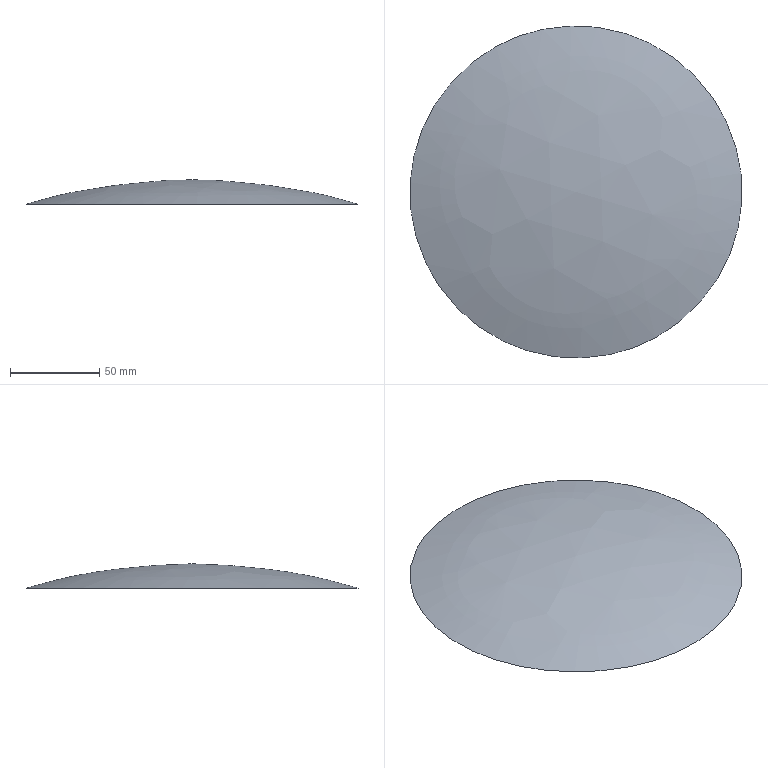Part | STEP file | 111_4 | 1 solid | 2 faces | box 185.942 x 185.942 x 13.599 mm | volume 185950 mm3 | spline 1 | plane 1
STEP:
#1=CARTESIAN_POINT('',(0.,0.,0.));
#2=DIRECTION('',(0.,0.,1.));
#3=DIRECTION('',(1.,0.,0.));
#4=AXIS2_PLACEMENT_3D('',#1,#2,#3);
#5=CARTESIAN_POINT('',(-44.573,81.59,-4.741));
#6=VERTEX_POINT('',#5);
#7=CARTESIAN_POINT('',(44.573,-81.59,-4.741));
#8=VERTEX_POINT('',#7);
#9=CARTESIAN_POINT('',(-44.573,81.59,-4.741));
#10=CARTESIAN_POINT('',(-47.267,80.117,-4.741));
#11=CARTESIAN_POINT('',(-49.867,78.524,-4.741));
#12=CARTESIAN_POINT('',(-54.882,75.105,-4.741));
#13=CARTESIAN_POINT('',(-57.297,73.279,-4.741));
#14=CARTESIAN_POINT('',(-61.944,69.395,-4.741));
#15=CARTESIAN_POINT('',(-64.176,67.337,-4.741));
#16=CARTESIAN_POINT('',(-67.384,64.073,-4.741));
#17=CARTESIAN_POINT('',(-68.431,62.953,-4.741));
#18=CARTESIAN_POINT('',(-70.471,60.661,-4.741));
#19=CARTESIAN_POINT('',(-71.458,59.495,-4.741));
#20=CARTESIAN_POINT('',(-74.324,55.936,-4.741));
#21=CARTESIAN_POINT('',(-76.108,53.482,-4.741));
#22=CARTESIAN_POINT('',(-79.426,48.417,-4.741));
#23=CARTESIAN_POINT('',(-80.961,45.806,-4.741));
#24=CARTESIAN_POINT('',(-83.074,41.769,-4.741));
#25=CARTESIAN_POINT('',(-83.746,40.404,-4.741));
#26=CARTESIAN_POINT('',(-84.708,38.325,-4.741));
#27=CARTESIAN_POINT('',(-85.02,37.627,-4.741));
#28=CARTESIAN_POINT('',(-85.629,36.221,-4.741));
#29=CARTESIAN_POINT('',(-85.925,35.511,-4.741));
#30=CARTESIAN_POINT('',(-87.359,31.959,-4.741));
#31=CARTESIAN_POINT('',(-88.357,29.083,-4.741));
#32=CARTESIAN_POINT('',(-90.064,23.264,-4.741));
#33=CARTESIAN_POINT('',(-90.774,20.321,-4.741));
#34=CARTESIAN_POINT('',(-91.904,14.368,-4.741));
#35=CARTESIAN_POINT('',(-92.325,11.358,-4.741));
#36=CARTESIAN_POINT('',(-92.735,6.792,-4.741));
#37=CARTESIAN_POINT('',(-92.835,5.258,-4.741));
#38=CARTESIAN_POINT('',(-92.958,2.198,-4.741));
#39=CARTESIAN_POINT('',(-92.981,0.673,-4.741));
#40=CARTESIAN_POINT('',(-92.939,-3.891,-4.741));
#41=CARTESIAN_POINT('',(-92.763,-6.917,-4.741));
#42=CARTESIAN_POINT('',(-92.116,-12.937,-4.741));
#43=CARTESIAN_POINT('',(-91.646,-15.93,-4.741));
#44=CARTESIAN_POINT('',(-90.719,-20.396,-4.741));
#45=CARTESIAN_POINT('',(-90.372,-21.881,-4.741));
#46=CARTESIAN_POINT('',(-89.604,-24.842,-4.741));
#47=CARTESIAN_POINT('',(-89.18,-26.321,-4.741));
#48=CARTESIAN_POINT('',(-87.809,-30.699,-4.741));
#49=CARTESIAN_POINT('',(-86.758,-33.553,-4.741));
#50=CARTESIAN_POINT('',(-84.389,-39.131,-4.741));
#51=CARTESIAN_POINT('',(-83.071,-41.856,-4.741));
#52=CARTESIAN_POINT('',(-80.168,-47.179,-4.741));
#53=CARTESIAN_POINT('',(-78.583,-49.776,-4.741));
#54=CARTESIAN_POINT('',(-75.999,-53.572,-4.741));
#55=CARTESIAN_POINT('',(-75.103,-54.822,-4.741));
#56=CARTESIAN_POINT('',(-73.261,-57.261,-4.741));
#57=CARTESIAN_POINT('',(-72.313,-58.453,-4.741));
#58=CARTESIAN_POINT('',(-69.389,-61.951,-4.741));
#59=CARTESIAN_POINT('',(-67.335,-64.177,-4.741));
#60=CARTESIAN_POINT('',(-63.017,-68.422,-4.741));
#61=CARTESIAN_POINT('',(-60.754,-70.44,-4.741));
#62=CARTESIAN_POINT('',(-57.2,-73.308,-4.741));
#63=CARTESIAN_POINT('',(-55.989,-74.237,-4.741));
#64=CARTESIAN_POINT('',(-54.131,-75.591,-4.741));
#65=CARTESIAN_POINT('',(-53.504,-76.036,-4.741));
#66=CARTESIAN_POINT('',(-52.244,-76.907,-4.741));
#67=CARTESIAN_POINT('',(-51.61,-77.334,-4.741));
#68=CARTESIAN_POINT('',(-48.418,-79.427,-4.741));
#69=CARTESIAN_POINT('',(-45.798,-80.965,-4.741));
#70=CARTESIAN_POINT('',(-40.431,-83.774,-4.741));
#71=CARTESIAN_POINT('',(-37.684,-85.046,-4.741));
#72=CARTESIAN_POINT('',(-32.06,-87.321,-4.741));
#73=CARTESIAN_POINT('',(-29.183,-88.325,-4.741));
#74=CARTESIAN_POINT('',(-24.769,-89.624,-4.741));
#75=CARTESIAN_POINT('',(-23.288,-90.02,-4.741));
#76=CARTESIAN_POINT('',(-20.322,-90.736,-4.741));
#77=CARTESIAN_POINT('',(-18.834,-91.056,-4.741));
#78=CARTESIAN_POINT('',(-14.36,-91.905,-4.741));
#79=CARTESIAN_POINT('',(-11.361,-92.324,-4.741));
#80=CARTESIAN_POINT('',(-5.33,-92.867,-4.741));
#81=CARTESIAN_POINT('',(-2.298,-92.993,-4.741));
#82=CARTESIAN_POINT('',(2.276,-92.956,-4.741));
#83=CARTESIAN_POINT('',(3.804,-92.906,-4.741));
#84=CARTESIAN_POINT('',(6.87,-92.729,-4.741));
#85=CARTESIAN_POINT('',(8.394,-92.604,-4.741));
#86=CARTESIAN_POINT('',(12.941,-92.116,-4.741));
#87=CARTESIAN_POINT('',(15.939,-91.644,-4.741));
#88=CARTESIAN_POINT('',(21.868,-90.413,-4.741));
#89=CARTESIAN_POINT('',(24.8,-89.654,-4.741));
#90=CARTESIAN_POINT('',(29.147,-88.297,-4.741));
#91=CARTESIAN_POINT('',(30.588,-87.808,-4.741));
#92=CARTESIAN_POINT('',(33.452,-86.757,-4.741));
#93=CARTESIAN_POINT('',(34.878,-86.194,-4.741));
#94=CARTESIAN_POINT('',(39.117,-84.397,-4.741));
#95=CARTESIAN_POINT('',(41.878,-83.062,-4.741));
#96=CARTESIAN_POINT('',(44.573,-81.59,-4.741));
#97=B_SPLINE_CURVE_WITH_KNOTS('',3,(#9,#10,#11,#12,#13,#14,#15,#16,#17,#18,#19,#20,#21,#22,#23,#24,#25,#26,#27,#28,#29,#30,#31,#32,#33,#34,#35,#36,#37,#38,#39,#40,#41,#42,#43,#44,#45,#46,#47,#48,#49,#50,#51,#52,#53,#54,#55,#56,#57,#58,#59,#60,#61,#62,#63,#64,#65,#66,#67,#68,#69,#70,#71,#72,#73,#74,#75,#76,#77,#78,#79,#80,#81,#82,#83,#84,#85,#86,#87,#88,#89,#90,#91,#92,#93,#94,#95,#96),.UNSPECIFIED.,.F.,.F.,(4,2,2,2,2,2,2,2,2,2,2,2,2,2,2,2,2,2,2,2,2,2,2,2,2,2,2,2,2,2,2,2,2,2,2,2,2,2,2,2,2,2,2,4),(0.,0.009082,0.01816,0.02724,0.03179,0.03633,0.04541,0.05449,0.05903,0.0613,0.06357,0.07265,0.08173,0.09082,0.09536,0.0999,0.109,0.1181,0.1226,0.1271,0.1362,0.1453,0.1544,0.1589,0.1635,0.1725,0.1816,0.1862,0.1884,0.1907,0.1998,0.2089,0.218,0.2225,0.227,0.2361,0.2452,0.2497,0.2543,0.2634,0.2724,0.277,0.2815,0.2906),.UNSPECIFIED.);
#98=CARTESIAN_POINT('',(124.544,-39.136,-18.55));
#99=CARTESIAN_POINT('',(72.365,-67.641,-0.438));
#100=CARTESIAN_POINT('',(17.819,-97.44,-0.438));
#101=CARTESIAN_POINT('',(-34.36,-125.945,-18.55));
#102=CARTESIAN_POINT('',(99.708,17.694,-0.6593));
#103=CARTESIAN_POINT('',(44.388,-12.527,18.543));
#104=CARTESIAN_POINT('',(-13.442,-44.12,18.543));
#105=CARTESIAN_POINT('',(-68.762,-74.341,-0.6593));
#106=CARTESIAN_POINT('',(68.762,74.341,-0.6593));
#107=CARTESIAN_POINT('',(13.442,44.12,18.543));
#108=CARTESIAN_POINT('',(-44.388,12.527,18.543));
#109=CARTESIAN_POINT('',(-99.708,-17.694,-0.6593));
#110=CARTESIAN_POINT('',(34.36,125.945,-18.55));
#111=CARTESIAN_POINT('',(-17.819,97.44,-0.438));
#112=CARTESIAN_POINT('',(-72.365,67.641,-0.438));
#113=CARTESIAN_POINT('',(-124.544,39.136,-18.55));
#114=(BOUNDED_SURFACE()B_SPLINE_SURFACE(3,3,((#98,#99,#100,#101),(#102,#103,#104,#105),(#106,#107,#108,#109),(#110,#111,#112,#113)),.UNSPECIFIED.,.F.,.F.,.F.)B_SPLINE_SURFACE_WITH_KNOTS((4,4),(4,4),(0.,1.),(0.,1.),.PIECEWISE_BEZIER_KNOTS.)GEOMETRIC_REPRESENTATION_ITEM()RATIONAL_B_SPLINE_SURFACE(((1.,0.9711,0.9711,1.),(0.9714,0.9433,0.9433,0.9714),(0.9714,0.9433,0.9433,0.9714),(1.,0.9711,0.9711,1.)))REPRESENTATION_ITEM('')SURFACE());
#115=CARTESIAN_POINT('',(0.994,0.5));
#116=CARTESIAN_POINT('',(0.994,0.503));
#117=CARTESIAN_POINT('',(0.9939,0.509));
#118=CARTESIAN_POINT('',(0.9937,0.518));
#119=CARTESIAN_POINT('',(0.9933,0.527));
#120=CARTESIAN_POINT('',(0.9927,0.5359));
#121=CARTESIAN_POINT('',(0.9919,0.5449));
#122=CARTESIAN_POINT('',(0.991,0.5537));
#123=CARTESIAN_POINT('',(0.99,0.5626));
#124=CARTESIAN_POINT('',(0.9888,0.5714));
#125=CARTESIAN_POINT('',(0.9874,0.5802));
#126=CARTESIAN_POINT('',(0.9858,0.589));
#127=CARTESIAN_POINT('',(0.9841,0.5977));
#128=CARTESIAN_POINT('',(0.9823,0.6064));
#129=CARTESIAN_POINT('',(0.9803,0.6151));
#130=CARTESIAN_POINT('',(0.9781,0.6238));
#131=CARTESIAN_POINT('',(0.9757,0.6324));
#132=CARTESIAN_POINT('',(0.9732,0.6409));
#133=CARTESIAN_POINT('',(0.9706,0.6495));
#134=CARTESIAN_POINT('',(0.9678,0.658));
#135=CARTESIAN_POINT('',(0.9648,0.6665));
#136=CARTESIAN_POINT('',(0.9616,0.6749));
#137=CARTESIAN_POINT('',(0.9583,0.6833));
#138=CARTESIAN_POINT('',(0.9549,0.6915));
#139=CARTESIAN_POINT('',(0.9514,0.6997));
#140=CARTESIAN_POINT('',(0.9477,0.7077));
#141=CARTESIAN_POINT('',(0.9438,0.7157));
#142=CARTESIAN_POINT('',(0.9398,0.7236));
#143=CARTESIAN_POINT('',(0.9357,0.7315));
#144=CARTESIAN_POINT('',(0.9315,0.7392));
#145=CARTESIAN_POINT('',(0.9271,0.7469));
#146=CARTESIAN_POINT('',(0.9225,0.7545));
#147=CARTESIAN_POINT('',(0.9179,0.762));
#148=CARTESIAN_POINT('',(0.9131,0.7694));
#149=CARTESIAN_POINT('',(0.9082,0.7767));
#150=CARTESIAN_POINT('',(0.9031,0.7839));
#151=CARTESIAN_POINT('',(0.8979,0.7911));
#152=CARTESIAN_POINT('',(0.8925,0.7982));
#153=CARTESIAN_POINT('',(0.8871,0.8052));
#154=CARTESIAN_POINT('',(0.8815,0.8121));
#155=CARTESIAN_POINT('',(0.8757,0.8189));
#156=CARTESIAN_POINT('',(0.8699,0.8255));
#157=CARTESIAN_POINT('',(0.864,0.8321));
#158=CARTESIAN_POINT('',(0.8579,0.8385));
#159=CARTESIAN_POINT('',(0.8518,0.8448));
#160=CARTESIAN_POINT('',(0.8456,0.851));
#161=CARTESIAN_POINT('',(0.8392,0.857));
#162=CARTESIAN_POINT('',(0.8328,0.8629));
#163=CARTESIAN_POINT('',(0.8263,0.8687));
#164=CARTESIAN_POINT('',(0.8197,0.8744));
#165=CARTESIAN_POINT('',(0.813,0.88));
#166=CARTESIAN_POINT('',(0.8062,0.8854));
#167=CARTESIAN_POINT('',(0.7992,0.8908));
#168=CARTESIAN_POINT('',(0.7922,0.896));
#169=CARTESIAN_POINT('',(0.7851,0.901));
#170=CARTESIAN_POINT('',(0.7779,0.906));
#171=CARTESIAN_POINT('',(0.7706,0.9109));
#172=CARTESIAN_POINT('',(0.7632,0.9156));
#173=CARTESIAN_POINT('',(0.7557,0.9202));
#174=CARTESIAN_POINT('',(0.7482,0.9246));
#175=CARTESIAN_POINT('',(0.7406,0.9289));
#176=CARTESIAN_POINT('',(0.7329,0.9331));
#177=CARTESIAN_POINT('',(0.7252,0.9371));
#178=CARTESIAN_POINT('',(0.7174,0.941));
#179=CARTESIAN_POINT('',(0.7096,0.9447));
#180=CARTESIAN_POINT('',(0.7017,0.9483));
#181=CARTESIAN_POINT('',(0.6938,0.9517));
#182=CARTESIAN_POINT('',(0.6858,0.955));
#183=CARTESIAN_POINT('',(0.6778,0.9582));
#184=CARTESIAN_POINT('',(0.6697,0.9612));
#185=CARTESIAN_POINT('',(0.6615,0.9641));
#186=CARTESIAN_POINT('',(0.6533,0.9668));
#187=CARTESIAN_POINT('',(0.6451,0.9694));
#188=CARTESIAN_POINT('',(0.6368,0.9719));
#189=CARTESIAN_POINT('',(0.6285,0.9742));
#190=CARTESIAN_POINT('',(0.62,0.9764));
#191=CARTESIAN_POINT('',(0.6116,0.9784));
#192=CARTESIAN_POINT('',(0.6031,0.9803));
#193=CARTESIAN_POINT('',(0.5945,0.982));
#194=CARTESIAN_POINT('',(0.586,0.9836));
#195=CARTESIAN_POINT('',(0.5775,0.985));
#196=CARTESIAN_POINT('',(0.5689,0.9863));
#197=CARTESIAN_POINT('',(0.5604,0.9874));
#198=CARTESIAN_POINT('',(0.5518,0.9884));
#199=CARTESIAN_POINT('',(0.5432,0.9892));
#200=CARTESIAN_POINT('',(0.5347,0.9899));
#201=CARTESIAN_POINT('',(0.5261,0.9904));
#202=CARTESIAN_POINT('',(0.5175,0.9908));
#203=CARTESIAN_POINT('',(0.5089,0.991));
#204=CARTESIAN_POINT('',(0.5003,0.9911));
#205=CARTESIAN_POINT('',(0.4917,0.991));
#206=CARTESIAN_POINT('',(0.4831,0.9908));
#207=CARTESIAN_POINT('',(0.4745,0.9904));
#208=CARTESIAN_POINT('',(0.4659,0.9899));
#209=CARTESIAN_POINT('',(0.4572,0.9892));
#210=CARTESIAN_POINT('',(0.4486,0.9884));
#211=CARTESIAN_POINT('',(0.4399,0.9874));
#212=CARTESIAN_POINT('',(0.4313,0.9863));
#213=CARTESIAN_POINT('',(0.4227,0.985));
#214=CARTESIAN_POINT('',(0.4142,0.9836));
#215=CARTESIAN_POINT('',(0.4057,0.982));
#216=CARTESIAN_POINT('',(0.3972,0.9803));
#217=CARTESIAN_POINT('',(0.3888,0.9785));
#218=CARTESIAN_POINT('',(0.3804,0.9765));
#219=CARTESIAN_POINT('',(0.3721,0.9743));
#220=CARTESIAN_POINT('',(0.3638,0.972));
#221=CARTESIAN_POINT('',(0.3555,0.9696));
#222=CARTESIAN_POINT('',(0.3473,0.967));
#223=CARTESIAN_POINT('',(0.3391,0.9643));
#224=CARTESIAN_POINT('',(0.3309,0.9614));
#225=CARTESIAN_POINT('',(0.3228,0.9584));
#226=CARTESIAN_POINT('',(0.3147,0.9553));
#227=CARTESIAN_POINT('',(0.3067,0.9519));
#228=CARTESIAN_POINT('',(0.2987,0.9485));
#229=CARTESIAN_POINT('',(0.2907,0.9449));
#230=CARTESIAN_POINT('',(0.2828,0.9411));
#231=CARTESIAN_POINT('',(0.275,0.9372));
#232=CARTESIAN_POINT('',(0.2672,0.9332));
#233=CARTESIAN_POINT('',(0.2596,0.929));
#234=CARTESIAN_POINT('',(0.252,0.9247));
#235=CARTESIAN_POINT('',(0.2445,0.9203));
#236=CARTESIAN_POINT('',(0.2371,0.9158));
#237=CARTESIAN_POINT('',(0.2298,0.9111));
#238=CARTESIAN_POINT('',(0.2225,0.9063));
#239=CARTESIAN_POINT('',(0.2154,0.9014));
#240=CARTESIAN_POINT('',(0.2083,0.8963));
#241=CARTESIAN_POINT('',(0.2013,0.8912));
#242=CARTESIAN_POINT('',(0.1944,0.8858));
#243=CARTESIAN_POINT('',(0.1875,0.8804));
#244=CARTESIAN_POINT('',(0.1808,0.8748));
#245=CARTESIAN_POINT('',(0.1741,0.8691));
#246=CARTESIAN_POINT('',(0.1676,0.8633));
#247=CARTESIAN_POINT('',(0.1611,0.8573));
#248=CARTESIAN_POINT('',(0.1547,0.8512));
#249=CARTESIAN_POINT('',(0.1484,0.845));
#250=CARTESIAN_POINT('',(0.1422,0.8386));
#251=CARTESIAN_POINT('',(0.1361,0.8322));
#252=CARTESIAN_POINT('',(0.1302,0.8257));
#253=CARTESIAN_POINT('',(0.1244,0.819));
#254=CARTESIAN_POINT('',(0.1187,0.8123));
#255=CARTESIAN_POINT('',(0.1132,0.8055));
#256=CARTESIAN_POINT('',(0.1078,0.7986));
#257=CARTESIAN_POINT('',(0.1024,0.7916));
#258=CARTESIAN_POINT('',(0.09727,0.7844));
#259=CARTESIAN_POINT('',(0.09221,0.7772));
#260=CARTESIAN_POINT('',(0.08728,0.7699));
#261=CARTESIAN_POINT('',(0.08248,0.7625));
#262=CARTESIAN_POINT('',(0.0778,0.755));
#263=CARTESIAN_POINT('',(0.07325,0.7474));
#264=CARTESIAN_POINT('',(0.06883,0.7397));
#265=CARTESIAN_POINT('',(0.06454,0.7319));
#266=CARTESIAN_POINT('',(0.06038,0.724));
#267=CARTESIAN_POINT('',(0.05634,0.716));
#268=CARTESIAN_POINT('',(0.05245,0.708));
#269=CARTESIAN_POINT('',(0.04872,0.6998));
#270=CARTESIAN_POINT('',(0.04514,0.6916));
#271=CARTESIAN_POINT('',(0.04172,0.6834));
#272=CARTESIAN_POINT('',(0.03845,0.6751));
#273=CARTESIAN_POINT('',(0.03534,0.6668));
#274=CARTESIAN_POINT('',(0.03238,0.6584));
#275=CARTESIAN_POINT('',(0.02958,0.65));
#276=CARTESIAN_POINT('',(0.02693,0.6415));
#277=CARTESIAN_POINT('',(0.02443,0.633));
#278=CARTESIAN_POINT('',(0.02209,0.6244));
#279=CARTESIAN_POINT('',(0.0199,0.6158));
#280=CARTESIAN_POINT('',(0.01787,0.6071));
#281=CARTESIAN_POINT('',(0.016,0.5984));
#282=CARTESIAN_POINT('',(0.01428,0.5896));
#283=CARTESIAN_POINT('',(0.01272,0.5808));
#284=CARTESIAN_POINT('',(0.01131,0.5719));
#285=CARTESIAN_POINT('',(0.01007,0.563));
#286=CARTESIAN_POINT('',(0.008989,0.5541));
#287=CARTESIAN_POINT('',(0.008071,0.5451));
#288=CARTESIAN_POINT('',(0.007321,0.5361));
#289=CARTESIAN_POINT('',(0.006737,0.5271));
#290=CARTESIAN_POINT('',(0.00632,0.5181));
#291=CARTESIAN_POINT('',(0.006069,0.509));
#292=CARTESIAN_POINT('',(0.006014,0.503));
#293=CARTESIAN_POINT('',(0.006014,0.5));
#294=B_SPLINE_CURVE_WITH_KNOTS('',3,(#115,#116,#117,#118,#119,#120,#121,#122,#123,#124,#125,#126,#127,#128,#129,#130,#131,#132,#133,#134,#135,#136,#137,#138,#139,#140,#141,#142,#143,#144,#145,#146,#147,#148,#149,#150,#151,#152,#153,#154,#155,#156,#157,#158,#159,#160,#161,#162,#163,#164,#165,#166,#167,#168,#169,#170,#171,#172,#173,#174,#175,#176,#177,#178,#179,#180,#181,#182,#183,#184,#185,#186,#187,#188,#189,#190,#191,#192,#193,#194,#195,#196,#197,#198,#199,#200,#201,#202,#203,#204,#205,#206,#207,#208,#209,#210,#211,#212,#213,#214,#215,#216,#217,#218,#219,#220,#221,#222,#223,#224,#225,#226,#227,#228,#229,#230,#231,#232,#233,#234,#235,#236,#237,#238,#239,#240,#241,#242,#243,#244,#245,#246,#247,#248,#249,#250,#251,#252,#253,#254,#255,#256,#257,#258,#259,#260,#261,#262,#263,#264,#265,#266,#267,#268,#269,#270,#271,#272,#273,#274,#275,#276,#277,#278,#279,#280,#281,#282,#283,#284,#285,#286,#287,#288,#289,#290,#291,#292,#293),.UNSPECIFIED.,.F.,.F.,(4,1,1,1,1,1,1,1,1,1,1,1,1,1,1,1,1,1,1,1,1,1,1,1,1,1,1,1,1,1,1,1,1,1,1,1,1,1,1,1,1,1,1,1,1,1,1,1,1,1,1,1,1,1,1,1,1,1,1,1,1,1,1,1,1,1,1,1,1,1,1,1,1,1,1,1,1,1,1,1,1,1,1,1,1,1,1,1,1,1,1,1,1,1,1,1,1,1,1,1,1,1,1,1,1,1,1,1,1,1,1,1,1,1,1,1,1,1,1,1,1,1,1,1,1,1,1,1,1,1,1,1,1,1,1,1,1,1,1,1,1,1,1,1,1,1,1,1,1,1,1,1,1,1,1,1,1,1,1,1,1,1,1,1,1,1,1,1,1,1,1,1,1,1,1,1,4),(0.,0.001651,0.003302,0.004954,0.006605,0.008256,0.009907,0.01156,0.01321,0.01486,0.01651,0.01816,0.01981,0.02147,0.02312,0.02477,0.02642,0.02807,0.02972,0.03137,0.03302,0.03468,0.03633,0.03798,0.03963,0.04128,0.04293,0.04458,0.04623,0.04788,0.04954,0.05119,0.05284,0.05449,0.05614,0.05779,0.05944,0.06109,0.06275,0.0644,0.06605,0.0677,0.06935,0.071,0.07265,0.0743,0.07595,0.07761,0.07926,0.08091,0.08256,0.08421,0.08586,0.08751,0.08916,0.09082,0.09247,0.09412,0.09577,0.09742,0.09907,0.1007,0.1024,0.104,0.1057,0.1073,0.109,0.1106,0.1123,0.1139,0.1156,0.1172,0.1189,0.1205,0.1222,0.1238,0.1255,0.1271,0.1288,0.1304,0.1321,0.1337,0.1354,0.137,0.1387,0.1404,0.142,0.1437,0.1453,0.147,0.1486,0.1503,0.1519,0.1536,0.1552,0.1569,0.1585,0.1602,0.1618,0.1635,0.1651,0.1668,0.1684,0.1701,0.1717,0.1734,0.175,0.1767,0.1783,0.18,0.1816,0.1833,0.1849,0.1866,0.1882,0.1899,0.1915,0.1932,0.1948,0.1965,0.1981,0.1998,0.2014,0.2031,0.2047,0.2064,0.2081,0.2097,0.2114,0.213,0.2147,0.2163,0.218,0.2196,0.2213,0.2229,0.2246,0.2262,0.2279,0.2295,0.2312,0.2328,0.2345,0.2361,0.2378,0.2394,0.2411,0.2427,0.2444,0.246,0.2477,0.2493,0.251,0.2526,0.2543,0.2559,0.2576,0.2592,0.2609,0.2625,0.2642,0.2658,0.2675,0.2691,0.2708,0.2724,0.2741,0.2757,0.2774,0.2791,0.2807,0.2824,0.284,0.2857,0.2873,0.289,0.2906),.QUASI_UNIFORM_KNOTS.);
#295=(GEOMETRIC_REPRESENTATION_CONTEXT(2)PARAMETRIC_REPRESENTATION_CONTEXT()REPRESENTATION_CONTEXT('',''));
#296=DEFINITIONAL_REPRESENTATION('',(#294),#295);
#297=PCURVE('',#114,#296);
#298=CARTESIAN_POINT('',(0.,0.,-4.741));
#299=DIRECTION('',(0.,0.,1.));
#300=DIRECTION('',(1.,0.,0.));
#301=AXIS2_PLACEMENT_3D('',#298,#299,#300);
#302=PLANE('',#301);
#303=CARTESIAN_POINT('',(-44.573,81.59));
#304=CARTESIAN_POINT('',(-47.267,80.117));
#305=CARTESIAN_POINT('',(-49.867,78.524));
#306=CARTESIAN_POINT('',(-54.882,75.105));
#307=CARTESIAN_POINT('',(-57.297,73.279));
#308=CARTESIAN_POINT('',(-61.944,69.395));
#309=CARTESIAN_POINT('',(-64.176,67.337));
#310=CARTESIAN_POINT('',(-67.384,64.073));
#311=CARTESIAN_POINT('',(-68.431,62.953));
#312=CARTESIAN_POINT('',(-70.471,60.661));
#313=CARTESIAN_POINT('',(-71.458,59.495));
#314=CARTESIAN_POINT('',(-74.324,55.936));
#315=CARTESIAN_POINT('',(-76.108,53.482));
#316=CARTESIAN_POINT('',(-79.426,48.417));
#317=CARTESIAN_POINT('',(-80.961,45.806));
#318=CARTESIAN_POINT('',(-83.074,41.769));
#319=CARTESIAN_POINT('',(-83.746,40.404));
#320=CARTESIAN_POINT('',(-84.708,38.325));
#321=CARTESIAN_POINT('',(-85.02,37.627));
#322=CARTESIAN_POINT('',(-85.629,36.221));
#323=CARTESIAN_POINT('',(-85.925,35.511));
#324=CARTESIAN_POINT('',(-87.359,31.959));
#325=CARTESIAN_POINT('',(-88.357,29.083));
#326=CARTESIAN_POINT('',(-90.064,23.264));
#327=CARTESIAN_POINT('',(-90.774,20.321));
#328=CARTESIAN_POINT('',(-91.904,14.368));
#329=CARTESIAN_POINT('',(-92.325,11.358));
#330=CARTESIAN_POINT('',(-92.735,6.792));
#331=CARTESIAN_POINT('',(-92.835,5.258));
#332=CARTESIAN_POINT('',(-92.958,2.198));
#333=CARTESIAN_POINT('',(-92.981,0.673));
#334=CARTESIAN_POINT('',(-92.939,-3.891));
#335=CARTESIAN_POINT('',(-92.763,-6.917));
#336=CARTESIAN_POINT('',(-92.116,-12.937));
#337=CARTESIAN_POINT('',(-91.646,-15.93));
#338=CARTESIAN_POINT('',(-90.719,-20.396));
#339=CARTESIAN_POINT('',(-90.372,-21.881));
#340=CARTESIAN_POINT('',(-89.604,-24.842));
#341=CARTESIAN_POINT('',(-89.18,-26.321));
#342=CARTESIAN_POINT('',(-87.809,-30.699));
#343=CARTESIAN_POINT('',(-86.758,-33.553));
#344=CARTESIAN_POINT('',(-84.389,-39.131));
#345=CARTESIAN_POINT('',(-83.071,-41.856));
#346=CARTESIAN_POINT('',(-80.168,-47.179));
#347=CARTESIAN_POINT('',(-78.583,-49.776));
#348=CARTESIAN_POINT('',(-75.999,-53.572));
#349=CARTESIAN_POINT('',(-75.103,-54.822));
#350=CARTESIAN_POINT('',(-73.261,-57.261));
#351=CARTESIAN_POINT('',(-72.313,-58.453));
#352=CARTESIAN_POINT('',(-69.389,-61.951));
#353=CARTESIAN_POINT('',(-67.335,-64.177));
#354=CARTESIAN_POINT('',(-63.017,-68.422));
#355=CARTESIAN_POINT('',(-60.754,-70.44));
#356=CARTESIAN_POINT('',(-57.2,-73.308));
#357=CARTESIAN_POINT('',(-55.989,-74.237));
#358=CARTESIAN_POINT('',(-54.131,-75.591));
#359=CARTESIAN_POINT('',(-53.504,-76.036));
#360=CARTESIAN_POINT('',(-52.244,-76.907));
#361=CARTESIAN_POINT('',(-51.61,-77.334));
#362=CARTESIAN_POINT('',(-48.418,-79.427));
#363=CARTESIAN_POINT('',(-45.798,-80.965));
#364=CARTESIAN_POINT('',(-40.431,-83.774));
#365=CARTESIAN_POINT('',(-37.684,-85.046));
#366=CARTESIAN_POINT('',(-32.06,-87.321));
#367=CARTESIAN_POINT('',(-29.183,-88.325));
#368=CARTESIAN_POINT('',(-24.769,-89.624));
#369=CARTESIAN_POINT('',(-23.288,-90.02));
#370=CARTESIAN_POINT('',(-20.322,-90.736));
#371=CARTESIAN_POINT('',(-18.834,-91.056));
#372=CARTESIAN_POINT('',(-14.36,-91.905));
#373=CARTESIAN_POINT('',(-11.361,-92.324));
#374=CARTESIAN_POINT('',(-5.33,-92.867));
#375=CARTESIAN_POINT('',(-2.298,-92.993));
#376=CARTESIAN_POINT('',(2.276,-92.956));
#377=CARTESIAN_POINT('',(3.804,-92.906));
#378=CARTESIAN_POINT('',(6.87,-92.729));
#379=CARTESIAN_POINT('',(8.394,-92.604));
#380=CARTESIAN_POINT('',(12.941,-92.116));
#381=CARTESIAN_POINT('',(15.939,-91.644));
#382=CARTESIAN_POINT('',(21.868,-90.413));
#383=CARTESIAN_POINT('',(24.8,-89.654));
#384=CARTESIAN_POINT('',(29.147,-88.297));
#385=CARTESIAN_POINT('',(30.588,-87.808));
#386=CARTESIAN_POINT('',(33.452,-86.757));
#387=CARTESIAN_POINT('',(34.878,-86.194));
#388=CARTESIAN_POINT('',(39.117,-84.397));
#389=CARTESIAN_POINT('',(41.878,-83.062));
#390=CARTESIAN_POINT('',(44.573,-81.59));
#391=B_SPLINE_CURVE_WITH_KNOTS('',3,(#303,#304,#305,#306,#307,#308,#309,#310,#311,#312,#313,#314,#315,#316,#317,#318,#319,#320,#321,#322,#323,#324,#325,#326,#327,#328,#329,#330,#331,#332,#333,#334,#335,#336,#337,#338,#339,#340,#341,#342,#343,#344,#345,#346,#347,#348,#349,#350,#351,#352,#353,#354,#355,#356,#357,#358,#359,#360,#361,#362,#363,#364,#365,#366,#367,#368,#369,#370,#371,#372,#373,#374,#375,#376,#377,#378,#379,#380,#381,#382,#383,#384,#385,#386,#387,#388,#389,#390),.UNSPECIFIED.,.F.,.F.,(4,2,2,2,2,2,2,2,2,2,2,2,2,2,2,2,2,2,2,2,2,2,2,2,2,2,2,2,2,2,2,2,2,2,2,2,2,2,2,2,2,2,2,4),(0.,0.009082,0.01816,0.02724,0.03179,0.03633,0.04541,0.05449,0.05903,0.0613,0.06357,0.07265,0.08173,0.09082,0.09536,0.0999,0.109,0.1181,0.1226,0.1271,0.1362,0.1453,0.1544,0.1589,0.1635,0.1725,0.1816,0.1862,0.1884,0.1907,0.1998,0.2089,0.218,0.2225,0.227,0.2361,0.2452,0.2497,0.2543,0.2634,0.2724,0.277,0.2815,0.2906),.UNSPECIFIED.);
#392=(GEOMETRIC_REPRESENTATION_CONTEXT(2)PARAMETRIC_REPRESENTATION_CONTEXT()REPRESENTATION_CONTEXT('',''));
#393=DEFINITIONAL_REPRESENTATION('',(#391),#392);
#394=PCURVE('',#302,#393);
#395=SURFACE_CURVE('',#97,(#297,#394),.PCURVE_S1.);
#396=EDGE_CURVE('',#6,#8,#395,.T.);
#397=ORIENTED_EDGE('',*,*,#396,.T.);
#398=CARTESIAN_POINT('',(44.573,-81.59,-4.741));
#399=CARTESIAN_POINT('',(47.267,-80.117,-4.741));
#400=CARTESIAN_POINT('',(49.867,-78.524,-4.741));
#401=CARTESIAN_POINT('',(54.882,-75.105,-4.741));
#402=CARTESIAN_POINT('',(57.297,-73.279,-4.741));
#403=CARTESIAN_POINT('',(61.944,-69.395,-4.741));
#404=CARTESIAN_POINT('',(64.176,-67.337,-4.741));
#405=CARTESIAN_POINT('',(67.384,-64.073,-4.741));
#406=CARTESIAN_POINT('',(68.431,-62.953,-4.741));
#407=CARTESIAN_POINT('',(70.471,-60.661,-4.741));
#408=CARTESIAN_POINT('',(71.458,-59.495,-4.741));
#409=CARTESIAN_POINT('',(74.324,-55.936,-4.741));
#410=CARTESIAN_POINT('',(76.108,-53.482,-4.741));
#411=CARTESIAN_POINT('',(79.426,-48.417,-4.741));
#412=CARTESIAN_POINT('',(80.961,-45.806,-4.741));
#413=CARTESIAN_POINT('',(83.074,-41.769,-4.741));
#414=CARTESIAN_POINT('',(83.746,-40.404,-4.741));
#415=CARTESIAN_POINT('',(84.708,-38.325,-4.741));
#416=CARTESIAN_POINT('',(85.02,-37.627,-4.741));
#417=CARTESIAN_POINT('',(85.629,-36.221,-4.741));
#418=CARTESIAN_POINT('',(85.925,-35.511,-4.741));
#419=CARTESIAN_POINT('',(87.359,-31.959,-4.741));
#420=CARTESIAN_POINT('',(88.357,-29.083,-4.741));
#421=CARTESIAN_POINT('',(90.064,-23.264,-4.741));
#422=CARTESIAN_POINT('',(90.774,-20.321,-4.741));
#423=CARTESIAN_POINT('',(91.904,-14.368,-4.741));
#424=CARTESIAN_POINT('',(92.325,-11.358,-4.741));
#425=CARTESIAN_POINT('',(92.735,-6.792,-4.741));
#426=CARTESIAN_POINT('',(92.835,-5.258,-4.741));
#427=CARTESIAN_POINT('',(92.958,-2.198,-4.741));
#428=CARTESIAN_POINT('',(92.981,-0.673,-4.741));
#429=CARTESIAN_POINT('',(92.939,3.891,-4.741));
#430=CARTESIAN_POINT('',(92.763,6.917,-4.741));
#431=CARTESIAN_POINT('',(92.116,12.937,-4.741));
#432=CARTESIAN_POINT('',(91.646,15.93,-4.741));
#433=CARTESIAN_POINT('',(90.719,20.396,-4.741));
#434=CARTESIAN_POINT('',(90.372,21.881,-4.741));
#435=CARTESIAN_POINT('',(89.604,24.842,-4.741));
#436=CARTESIAN_POINT('',(89.18,26.321,-4.741));
#437=CARTESIAN_POINT('',(87.809,30.699,-4.741));
#438=CARTESIAN_POINT('',(86.758,33.553,-4.741));
#439=CARTESIAN_POINT('',(84.389,39.131,-4.741));
#440=CARTESIAN_POINT('',(83.071,41.856,-4.741));
#441=CARTESIAN_POINT('',(80.168,47.179,-4.741));
#442=CARTESIAN_POINT('',(78.583,49.776,-4.741));
#443=CARTESIAN_POINT('',(75.999,53.572,-4.741));
#444=CARTESIAN_POINT('',(75.103,54.822,-4.741));
#445=CARTESIAN_POINT('',(73.261,57.261,-4.741));
#446=CARTESIAN_POINT('',(72.313,58.453,-4.741));
#447=CARTESIAN_POINT('',(69.389,61.951,-4.741));
#448=CARTESIAN_POINT('',(67.335,64.177,-4.741));
#449=CARTESIAN_POINT('',(63.017,68.422,-4.741));
#450=CARTESIAN_POINT('',(60.754,70.44,-4.741));
#451=CARTESIAN_POINT('',(57.2,73.308,-4.741));
#452=CARTESIAN_POINT('',(55.989,74.237,-4.741));
#453=CARTESIAN_POINT('',(54.131,75.591,-4.741));
#454=CARTESIAN_POINT('',(53.504,76.036,-4.741));
#455=CARTESIAN_POINT('',(52.244,76.907,-4.741));
#456=CARTESIAN_POINT('',(51.61,77.334,-4.741));
#457=CARTESIAN_POINT('',(48.418,79.427,-4.741));
#458=CARTESIAN_POINT('',(45.798,80.965,-4.741));
#459=CARTESIAN_POINT('',(40.431,83.774,-4.741));
#460=CARTESIAN_POINT('',(37.684,85.046,-4.741));
#461=CARTESIAN_POINT('',(32.06,87.321,-4.741));
#462=CARTESIAN_POINT('',(29.183,88.325,-4.741));
#463=CARTESIAN_POINT('',(24.769,89.624,-4.741));
#464=CARTESIAN_POINT('',(23.288,90.02,-4.741));
#465=CARTESIAN_POINT('',(20.322,90.736,-4.741));
#466=CARTESIAN_POINT('',(18.834,91.056,-4.741));
#467=CARTESIAN_POINT('',(14.36,91.905,-4.741));
#468=CARTESIAN_POINT('',(11.361,92.324,-4.741));
#469=CARTESIAN_POINT('',(5.33,92.867,-4.741));
#470=CARTESIAN_POINT('',(2.298,92.993,-4.741));
#471=CARTESIAN_POINT('',(-2.276,92.956,-4.741));
#472=CARTESIAN_POINT('',(-3.804,92.906,-4.741));
#473=CARTESIAN_POINT('',(-6.87,92.729,-4.741));
#474=CARTESIAN_POINT('',(-8.394,92.604,-4.741));
#475=CARTESIAN_POINT('',(-12.941,92.116,-4.741));
#476=CARTESIAN_POINT('',(-15.939,91.644,-4.741));
#477=CARTESIAN_POINT('',(-21.868,90.413,-4.741));
#478=CARTESIAN_POINT('',(-24.8,89.654,-4.741));
#479=CARTESIAN_POINT('',(-29.147,88.297,-4.741));
#480=CARTESIAN_POINT('',(-30.588,87.808,-4.741));
#481=CARTESIAN_POINT('',(-33.452,86.757,-4.741));
#482=CARTESIAN_POINT('',(-34.878,86.194,-4.741));
#483=CARTESIAN_POINT('',(-39.117,84.397,-4.741));
#484=CARTESIAN_POINT('',(-41.878,83.062,-4.741));
#485=CARTESIAN_POINT('',(-44.573,81.59,-4.741));
#486=B_SPLINE_CURVE_WITH_KNOTS('',3,(#398,#399,#400,#401,#402,#403,#404,#405,#406,#407,#408,#409,#410,#411,#412,#413,#414,#415,#416,#417,#418,#419,#420,#421,#422,#423,#424,#425,#426,#427,#428,#429,#430,#431,#432,#433,#434,#435,#436,#437,#438,#439,#440,#441,#442,#443,#444,#445,#446,#447,#448,#449,#450,#451,#452,#453,#454,#455,#456,#457,#458,#459,#460,#461,#462,#463,#464,#465,#466,#467,#468,#469,#470,#471,#472,#473,#474,#475,#476,#477,#478,#479,#480,#481,#482,#483,#484,#485),.UNSPECIFIED.,.F.,.F.,(4,2,2,2,2,2,2,2,2,2,2,2,2,2,2,2,2,2,2,2,2,2,2,2,2,2,2,2,2,2,2,2,2,2,2,2,2,2,2,2,2,2,2,4),(0.2906,0.2997,0.3088,0.3179,0.3224,0.3269,0.336,0.3451,0.3496,0.3519,0.3542,0.3633,0.3723,0.3814,0.386,0.3905,0.3996,0.4087,0.4132,0.4178,0.4268,0.4359,0.445,0.4495,0.4541,0.4632,0.4722,0.4768,0.4791,0.4813,0.4904,0.4995,0.5086,0.5131,0.5176,0.5267,0.5358,0.5404,0.5449,0.554,0.5631,0.5676,0.5721,0.5812),.UNSPECIFIED.);
#487=CARTESIAN_POINT('',(0.006014,0.5));
#488=CARTESIAN_POINT('',(0.006014,0.497));
#489=CARTESIAN_POINT('',(0.006069,0.491));
#490=CARTESIAN_POINT('',(0.006319,0.482));
#491=CARTESIAN_POINT('',(0.006733,0.473));
#492=CARTESIAN_POINT('',(0.00731,0.4641));
#493=CARTESIAN_POINT('',(0.008051,0.4551));
#494=CARTESIAN_POINT('',(0.008952,0.4463));
#495=CARTESIAN_POINT('',(0.01001,0.4374));
#496=CARTESIAN_POINT('',(0.01124,0.4286));
#497=CARTESIAN_POINT('',(0.01262,0.4198));
#498=CARTESIAN_POINT('',(0.01416,0.411));
#499=CARTESIAN_POINT('',(0.01586,0.4023));
#500=CARTESIAN_POINT('',(0.01772,0.3936));
#501=CARTESIAN_POINT('',(0.01974,0.3849));
#502=CARTESIAN_POINT('',(0.02192,0.3762));
#503=CARTESIAN_POINT('',(0.02426,0.3676));
#504=CARTESIAN_POINT('',(0.02676,0.3591));
#505=CARTESIAN_POINT('',(0.02942,0.3505));
#506=CARTESIAN_POINT('',(0.03225,0.342));
#507=CARTESIAN_POINT('',(0.03523,0.3335));
#508=CARTESIAN_POINT('',(0.03837,0.3251));
#509=CARTESIAN_POINT('',(0.04166,0.3167));
#510=CARTESIAN_POINT('',(0.04508,0.3085));
#511=CARTESIAN_POINT('',(0.04864,0.3003));
#512=CARTESIAN_POINT('',(0.05235,0.2923));
#513=CARTESIAN_POINT('',(0.05619,0.2843));
#514=CARTESIAN_POINT('',(0.06017,0.2764));
#515=CARTESIAN_POINT('',(0.06429,0.2685));
#516=CARTESIAN_POINT('',(0.06854,0.2608));
#517=CARTESIAN_POINT('',(0.07293,0.2531));
#518=CARTESIAN_POINT('',(0.07746,0.2455));
#519=CARTESIAN_POINT('',(0.08212,0.238));
#520=CARTESIAN_POINT('',(0.08691,0.2306));
#521=CARTESIAN_POINT('',(0.09185,0.2233));
#522=CARTESIAN_POINT('',(0.09691,0.2161));
#523=CARTESIAN_POINT('',(0.1021,0.2089));
#524=CARTESIAN_POINT('',(0.1075,0.2018));
#525=CARTESIAN_POINT('',(0.1129,0.1948));
#526=CARTESIAN_POINT('',(0.1185,0.1879));
#527=CARTESIAN_POINT('',(0.1243,0.1811));
#528=CARTESIAN_POINT('',(0.1301,0.1745));
#529=CARTESIAN_POINT('',(0.136,0.1679));
#530=CARTESIAN_POINT('',(0.1421,0.1615));
#531=CARTESIAN_POINT('',(0.1482,0.1552));
#532=CARTESIAN_POINT('',(0.1544,0.149));
#533=CARTESIAN_POINT('',(0.1608,0.143));
#534=CARTESIAN_POINT('',(0.1672,0.1371));
#535=CARTESIAN_POINT('',(0.1737,0.1313));
#536=CARTESIAN_POINT('',(0.1803,0.1256));
#537=CARTESIAN_POINT('',(0.187,0.12));
#538=CARTESIAN_POINT('',(0.1938,0.1146));
#539=CARTESIAN_POINT('',(0.2008,0.1092));
#540=CARTESIAN_POINT('',(0.2078,0.104));
#541=CARTESIAN_POINT('',(0.2149,0.09895));
#542=CARTESIAN_POINT('',(0.2221,0.09399));
#543=CARTESIAN_POINT('',(0.2294,0.08915));
#544=CARTESIAN_POINT('',(0.2368,0.08442));
#545=CARTESIAN_POINT('',(0.2443,0.07982));
#546=CARTESIAN_POINT('',(0.2518,0.07537));
#547=CARTESIAN_POINT('',(0.2594,0.07106));
#548=CARTESIAN_POINT('',(0.2671,0.0669));
#549=CARTESIAN_POINT('',(0.2748,0.06289));
#550=CARTESIAN_POINT('',(0.2826,0.05902));
#551=CARTESIAN_POINT('',(0.2904,0.05529));
#552=CARTESIAN_POINT('',(0.2983,0.05171));
#553=CARTESIAN_POINT('',(0.3062,0.04827));
#554=CARTESIAN_POINT('',(0.3142,0.04497));
#555=CARTESIAN_POINT('',(0.3222,0.04181));
#556=CARTESIAN_POINT('',(0.3303,0.03879));
#557=CARTESIAN_POINT('',(0.3385,0.03591));
#558=CARTESIAN_POINT('',(0.3467,0.03317));
#559=CARTESIAN_POINT('',(0.3549,0.03058));
#560=CARTESIAN_POINT('',(0.3632,0.02812));
#561=CARTESIAN_POINT('',(0.3715,0.02581));
#562=CARTESIAN_POINT('',(0.38,0.02364));
#563=CARTESIAN_POINT('',(0.3884,0.02161));
#564=CARTESIAN_POINT('',(0.3969,0.01973));
#565=CARTESIAN_POINT('',(0.4055,0.018));
#566=CARTESIAN_POINT('',(0.414,0.01642));
#567=CARTESIAN_POINT('',(0.4225,0.015));
#568=CARTESIAN_POINT('',(0.4311,0.01373));
#569=CARTESIAN_POINT('',(0.4396,0.0126));
#570=CARTESIAN_POINT('',(0.4482,0.01163));
#571=CARTESIAN_POINT('',(0.4568,0.01081));
#572=CARTESIAN_POINT('',(0.4653,0.01014));
#573=CARTESIAN_POINT('',(0.4739,0.009613));
#574=CARTESIAN_POINT('',(0.4825,0.009236));
#575=CARTESIAN_POINT('',(0.4911,0.009008));
#576=CARTESIAN_POINT('',(0.4997,0.008928));
#577=CARTESIAN_POINT('',(0.5083,0.008997));
#578=CARTESIAN_POINT('',(0.5169,0.009214));
#579=CARTESIAN_POINT('',(0.5255,0.009582));
#580=CARTESIAN_POINT('',(0.5341,0.0101));
#581=CARTESIAN_POINT('',(0.5428,0.01077));
#582=CARTESIAN_POINT('',(0.5514,0.0116));
#583=CARTESIAN_POINT('',(0.5601,0.01257));
#584=CARTESIAN_POINT('',(0.5687,0.0137));
#585=CARTESIAN_POINT('',(0.5773,0.01497));
#586=CARTESIAN_POINT('',(0.5858,0.01639));
#587=CARTESIAN_POINT('',(0.5943,0.01796));
#588=CARTESIAN_POINT('',(0.6028,0.01967));
#589=CARTESIAN_POINT('',(0.6112,0.02153));
#590=CARTESIAN_POINT('',(0.6196,0.02353));
#591=CARTESIAN_POINT('',(0.6279,0.02567));
#592=CARTESIAN_POINT('',(0.6362,0.02796));
#593=CARTESIAN_POINT('',(0.6445,0.0304));
#594=CARTESIAN_POINT('',(0.6527,0.03297));
#595=CARTESIAN_POINT('',(0.6609,0.0357));
#596=CARTESIAN_POINT('',(0.6691,0.03857));
#597=CARTESIAN_POINT('',(0.6772,0.04158));
#598=CARTESIAN_POINT('',(0.6853,0.04475));
#599=CARTESIAN_POINT('',(0.6933,0.04806));
#600=CARTESIAN_POINT('',(0.7013,0.05152));
#601=CARTESIAN_POINT('',(0.7093,0.05514));
#602=CARTESIAN_POINT('',(0.7172,0.05891));
#603=CARTESIAN_POINT('',(0.725,0.0628));
#604=CARTESIAN_POINT('',(0.7328,0.06683));
#605=CARTESIAN_POINT('',(0.7404,0.07098));
#606=CARTESIAN_POINT('',(0.748,0.07527));
#607=CARTESIAN_POINT('',(0.7555,0.07968));
#608=CARTESIAN_POINT('',(0.7629,0.08422));
#609=CARTESIAN_POINT('',(0.7702,0.08889));
#610=CARTESIAN_POINT('',(0.7775,0.09368));
#611=CARTESIAN_POINT('',(0.7846,0.09861));
#612=CARTESIAN_POINT('',(0.7917,0.1037));
#613=CARTESIAN_POINT('',(0.7987,0.1088));
#614=CARTESIAN_POINT('',(0.8056,0.1142));
#615=CARTESIAN_POINT('',(0.8125,0.1196));
#616=CARTESIAN_POINT('',(0.8192,0.1252));
#617=CARTESIAN_POINT('',(0.8259,0.1309));
#618=CARTESIAN_POINT('',(0.8324,0.1367));
#619=CARTESIAN_POINT('',(0.8389,0.1427));
#620=CARTESIAN_POINT('',(0.8453,0.1488));
#621=CARTESIAN_POINT('',(0.8516,0.155));
#622=CARTESIAN_POINT('',(0.8578,0.1614));
#623=CARTESIAN_POINT('',(0.8639,0.1678));
#624=CARTESIAN_POINT('',(0.8698,0.1743));
#625=CARTESIAN_POINT('',(0.8756,0.181));
#626=CARTESIAN_POINT('',(0.8813,0.1877));
#627=CARTESIAN_POINT('',(0.8868,0.1945));
#628=CARTESIAN_POINT('',(0.8922,0.2014));
#629=CARTESIAN_POINT('',(0.8976,0.2084));
#630=CARTESIAN_POINT('',(0.9027,0.2156));
#631=CARTESIAN_POINT('',(0.9078,0.2228));
#632=CARTESIAN_POINT('',(0.9127,0.2301));
#633=CARTESIAN_POINT('',(0.9175,0.2375));
#634=CARTESIAN_POINT('',(0.9222,0.245));
#635=CARTESIAN_POINT('',(0.9267,0.2526));
#636=CARTESIAN_POINT('',(0.9312,0.2603));
#637=CARTESIAN_POINT('',(0.9355,0.2681));
#638=CARTESIAN_POINT('',(0.9396,0.276));
#639=CARTESIAN_POINT('',(0.9437,0.284));
#640=CARTESIAN_POINT('',(0.9475,0.292));
#641=CARTESIAN_POINT('',(0.9513,0.3002));
#642=CARTESIAN_POINT('',(0.9549,0.3084));
#643=CARTESIAN_POINT('',(0.9583,0.3166));
#644=CARTESIAN_POINT('',(0.9615,0.3249));
#645=CARTESIAN_POINT('',(0.9647,0.3332));
#646=CARTESIAN_POINT('',(0.9676,0.3416));
#647=CARTESIAN_POINT('',(0.9704,0.35));
#648=CARTESIAN_POINT('',(0.9731,0.3585));
#649=CARTESIAN_POINT('',(0.9756,0.367));
#650=CARTESIAN_POINT('',(0.9779,0.3756));
#651=CARTESIAN_POINT('',(0.9801,0.3842));
#652=CARTESIAN_POINT('',(0.9821,0.3929));
#653=CARTESIAN_POINT('',(0.984,0.4016));
#654=CARTESIAN_POINT('',(0.9857,0.4104));
#655=CARTESIAN_POINT('',(0.9873,0.4192));
#656=CARTESIAN_POINT('',(0.9887,0.4281));
#657=CARTESIAN_POINT('',(0.9899,0.437));
#658=CARTESIAN_POINT('',(0.991,0.4459));
#659=CARTESIAN_POINT('',(0.9919,0.4549));
#660=CARTESIAN_POINT('',(0.9927,0.4639));
#661=CARTESIAN_POINT('',(0.9933,0.4729));
#662=CARTESIAN_POINT('',(0.9937,0.4819));
#663=CARTESIAN_POINT('',(0.9939,0.491));
#664=CARTESIAN_POINT('',(0.994,0.497));
#665=CARTESIAN_POINT('',(0.994,0.5));
#666=B_SPLINE_CURVE_WITH_KNOTS('',3,(#487,#488,#489,#490,#491,#492,#493,#494,#495,#496,#497,#498,#499,#500,#501,#502,#503,#504,#505,#506,#507,#508,#509,#510,#511,#512,#513,#514,#515,#516,#517,#518,#519,#520,#521,#522,#523,#524,#525,#526,#527,#528,#529,#530,#531,#532,#533,#534,#535,#536,#537,#538,#539,#540,#541,#542,#543,#544,#545,#546,#547,#548,#549,#550,#551,#552,#553,#554,#555,#556,#557,#558,#559,#560,#561,#562,#563,#564,#565,#566,#567,#568,#569,#570,#571,#572,#573,#574,#575,#576,#577,#578,#579,#580,#581,#582,#583,#584,#585,#586,#587,#588,#589,#590,#591,#592,#593,#594,#595,#596,#597,#598,#599,#600,#601,#602,#603,#604,#605,#606,#607,#608,#609,#610,#611,#612,#613,#614,#615,#616,#617,#618,#619,#620,#621,#622,#623,#624,#625,#626,#627,#628,#629,#630,#631,#632,#633,#634,#635,#636,#637,#638,#639,#640,#641,#642,#643,#644,#645,#646,#647,#648,#649,#650,#651,#652,#653,#654,#655,#656,#657,#658,#659,#660,#661,#662,#663,#664,#665),.UNSPECIFIED.,.F.,.F.,(4,1,1,1,1,1,1,1,1,1,1,1,1,1,1,1,1,1,1,1,1,1,1,1,1,1,1,1,1,1,1,1,1,1,1,1,1,1,1,1,1,1,1,1,1,1,1,1,1,1,1,1,1,1,1,1,1,1,1,1,1,1,1,1,1,1,1,1,1,1,1,1,1,1,1,1,1,1,1,1,1,1,1,1,1,1,1,1,1,1,1,1,1,1,1,1,1,1,1,1,1,1,1,1,1,1,1,1,1,1,1,1,1,1,1,1,1,1,1,1,1,1,1,1,1,1,1,1,1,1,1,1,1,1,1,1,1,1,1,1,1,1,1,1,1,1,1,1,1,1,1,1,1,1,1,1,1,1,1,1,1,1,1,1,1,1,1,1,1,1,1,1,1,1,1,1,4),(0.2906,0.2923,0.2939,0.2956,0.2972,0.2989,0.3005,0.3022,0.3038,0.3055,0.3071,0.3088,0.3104,0.3121,0.3137,0.3154,0.317,0.3187,0.3203,0.322,0.3236,0.3253,0.3269,0.3286,0.3302,0.3319,0.3335,0.3352,0.3368,0.3385,0.3401,0.3418,0.3434,0.3451,0.3468,0.3484,0.3501,0.3517,0.3534,0.355,0.3567,0.3583,0.36,0.3616,0.3633,0.3649,0.3666,0.3682,0.3699,0.3715,0.3732,0.3748,0.3765,0.3781,0.3798,0.3814,0.3831,0.3847,0.3864,0.388,0.3897,0.3913,0.393,0.3946,0.3963,0.3979,0.3996,0.4012,0.4029,0.4045,0.4062,0.4078,0.4095,0.4111,0.4128,0.4144,0.4161,0.4178,0.4194,0.4211,0.4227,0.4244,0.426,0.4277,0.4293,0.431,0.4326,0.4343,0.4359,0.4376,0.4392,0.4409,0.4425,0.4442,0.4458,0.4475,0.4491,0.4508,0.4524,0.4541,0.4557,0.4574,0.459,0.4607,0.4623,0.464,0.4656,0.4673,0.4689,0.4706,0.4722,0.4739,0.4755,0.4772,0.4788,0.4805,0.4821,0.4838,0.4855,0.4871,0.4888,0.4904,0.4921,0.4937,0.4954,0.497,0.4987,0.5003,0.502,0.5036,0.5053,0.5069,0.5086,0.5102,0.5119,0.5135,0.5152,0.5168,0.5185,0.5201,0.5218,0.5234,0.5251,0.5267,0.5284,0.53,0.5317,0.5333,0.535,0.5366,0.5383,0.5399,0.5416,0.5432,0.5449,0.5465,0.5482,0.5498,0.5515,0.5531,0.5548,0.5565,0.5581,0.5598,0.5614,0.5631,0.5647,0.5664,0.568,0.5697,0.5713,0.573,0.5746,0.5763,0.5779,0.5796,0.5812),.QUASI_UNIFORM_KNOTS.);
#667=(GEOMETRIC_REPRESENTATION_CONTEXT(2)PARAMETRIC_REPRESENTATION_CONTEXT()REPRESENTATION_CONTEXT('',''));
#668=DEFINITIONAL_REPRESENTATION('',(#666),#667);
#669=PCURVE('',#114,#668);
#670=CARTESIAN_POINT('',(44.573,-81.59));
#671=CARTESIAN_POINT('',(47.267,-80.117));
#672=CARTESIAN_POINT('',(49.867,-78.524));
#673=CARTESIAN_POINT('',(54.882,-75.105));
#674=CARTESIAN_POINT('',(57.297,-73.279));
#675=CARTESIAN_POINT('',(61.944,-69.395));
#676=CARTESIAN_POINT('',(64.176,-67.337));
#677=CARTESIAN_POINT('',(67.384,-64.073));
#678=CARTESIAN_POINT('',(68.431,-62.953));
#679=CARTESIAN_POINT('',(70.471,-60.661));
#680=CARTESIAN_POINT('',(71.458,-59.495));
#681=CARTESIAN_POINT('',(74.324,-55.936));
#682=CARTESIAN_POINT('',(76.108,-53.482));
#683=CARTESIAN_POINT('',(79.426,-48.417));
#684=CARTESIAN_POINT('',(80.961,-45.806));
#685=CARTESIAN_POINT('',(83.074,-41.769));
#686=CARTESIAN_POINT('',(83.746,-40.404));
#687=CARTESIAN_POINT('',(84.708,-38.325));
#688=CARTESIAN_POINT('',(85.02,-37.627));
#689=CARTESIAN_POINT('',(85.629,-36.221));
#690=CARTESIAN_POINT('',(85.925,-35.511));
#691=CARTESIAN_POINT('',(87.359,-31.959));
#692=CARTESIAN_POINT('',(88.357,-29.083));
#693=CARTESIAN_POINT('',(90.064,-23.264));
#694=CARTESIAN_POINT('',(90.774,-20.321));
#695=CARTESIAN_POINT('',(91.904,-14.368));
#696=CARTESIAN_POINT('',(92.325,-11.358));
#697=CARTESIAN_POINT('',(92.735,-6.792));
#698=CARTESIAN_POINT('',(92.835,-5.258));
#699=CARTESIAN_POINT('',(92.958,-2.198));
#700=CARTESIAN_POINT('',(92.981,-0.673));
#701=CARTESIAN_POINT('',(92.939,3.891));
#702=CARTESIAN_POINT('',(92.763,6.917));
#703=CARTESIAN_POINT('',(92.116,12.937));
#704=CARTESIAN_POINT('',(91.646,15.93));
#705=CARTESIAN_POINT('',(90.719,20.396));
#706=CARTESIAN_POINT('',(90.372,21.881));
#707=CARTESIAN_POINT('',(89.604,24.842));
#708=CARTESIAN_POINT('',(89.18,26.321));
#709=CARTESIAN_POINT('',(87.809,30.699));
#710=CARTESIAN_POINT('',(86.758,33.553));
#711=CARTESIAN_POINT('',(84.389,39.131));
#712=CARTESIAN_POINT('',(83.071,41.856));
#713=CARTESIAN_POINT('',(80.168,47.179));
#714=CARTESIAN_POINT('',(78.583,49.776));
#715=CARTESIAN_POINT('',(75.999,53.572));
#716=CARTESIAN_POINT('',(75.103,54.822));
#717=CARTESIAN_POINT('',(73.261,57.261));
#718=CARTESIAN_POINT('',(72.313,58.453));
#719=CARTESIAN_POINT('',(69.389,61.951));
#720=CARTESIAN_POINT('',(67.335,64.177));
#721=CARTESIAN_POINT('',(63.017,68.422));
#722=CARTESIAN_POINT('',(60.754,70.44));
#723=CARTESIAN_POINT('',(57.2,73.308));
#724=CARTESIAN_POINT('',(55.989,74.237));
#725=CARTESIAN_POINT('',(54.131,75.591));
#726=CARTESIAN_POINT('',(53.504,76.036));
#727=CARTESIAN_POINT('',(52.244,76.907));
#728=CARTESIAN_POINT('',(51.61,77.334));
#729=CARTESIAN_POINT('',(48.418,79.427));
#730=CARTESIAN_POINT('',(45.798,80.965));
#731=CARTESIAN_POINT('',(40.431,83.774));
#732=CARTESIAN_POINT('',(37.684,85.046));
#733=CARTESIAN_POINT('',(32.06,87.321));
#734=CARTESIAN_POINT('',(29.183,88.325));
#735=CARTESIAN_POINT('',(24.769,89.624));
#736=CARTESIAN_POINT('',(23.288,90.02));
#737=CARTESIAN_POINT('',(20.322,90.736));
#738=CARTESIAN_POINT('',(18.834,91.056));
#739=CARTESIAN_POINT('',(14.36,91.905));
#740=CARTESIAN_POINT('',(11.361,92.324));
#741=CARTESIAN_POINT('',(5.33,92.867));
#742=CARTESIAN_POINT('',(2.298,92.993));
#743=CARTESIAN_POINT('',(-2.276,92.956));
#744=CARTESIAN_POINT('',(-3.804,92.906));
#745=CARTESIAN_POINT('',(-6.87,92.729));
#746=CARTESIAN_POINT('',(-8.394,92.604));
#747=CARTESIAN_POINT('',(-12.941,92.116));
#748=CARTESIAN_POINT('',(-15.939,91.644));
#749=CARTESIAN_POINT('',(-21.868,90.413));
#750=CARTESIAN_POINT('',(-24.8,89.654));
#751=CARTESIAN_POINT('',(-29.147,88.297));
#752=CARTESIAN_POINT('',(-30.588,87.808));
#753=CARTESIAN_POINT('',(-33.452,86.757));
#754=CARTESIAN_POINT('',(-34.878,86.194));
#755=CARTESIAN_POINT('',(-39.117,84.397));
#756=CARTESIAN_POINT('',(-41.878,83.062));
#757=CARTESIAN_POINT('',(-44.573,81.59));
#758=B_SPLINE_CURVE_WITH_KNOTS('',3,(#670,#671,#672,#673,#674,#675,#676,#677,#678,#679,#680,#681,#682,#683,#684,#685,#686,#687,#688,#689,#690,#691,#692,#693,#694,#695,#696,#697,#698,#699,#700,#701,#702,#703,#704,#705,#706,#707,#708,#709,#710,#711,#712,#713,#714,#715,#716,#717,#718,#719,#720,#721,#722,#723,#724,#725,#726,#727,#728,#729,#730,#731,#732,#733,#734,#735,#736,#737,#738,#739,#740,#741,#742,#743,#744,#745,#746,#747,#748,#749,#750,#751,#752,#753,#754,#755,#756,#757),.UNSPECIFIED.,.F.,.F.,(4,2,2,2,2,2,2,2,2,2,2,2,2,2,2,2,2,2,2,2,2,2,2,2,2,2,2,2,2,2,2,2,2,2,2,2,2,2,2,2,2,2,2,4),(0.2906,0.2997,0.3088,0.3179,0.3224,0.3269,0.336,0.3451,0.3496,0.3519,0.3542,0.3633,0.3723,0.3814,0.386,0.3905,0.3996,0.4087,0.4132,0.4178,0.4268,0.4359,0.445,0.4495,0.4541,0.4632,0.4722,0.4768,0.4791,0.4813,0.4904,0.4995,0.5086,0.5131,0.5176,0.5267,0.5358,0.5404,0.5449,0.554,0.5631,0.5676,0.5721,0.5812),.UNSPECIFIED.);
#759=(GEOMETRIC_REPRESENTATION_CONTEXT(2)PARAMETRIC_REPRESENTATION_CONTEXT()REPRESENTATION_CONTEXT('',''));
#760=DEFINITIONAL_REPRESENTATION('',(#758),#759);
#761=PCURVE('',#302,#760);
#762=SURFACE_CURVE('',#486,(#669,#761),.PCURVE_S1.);
#763=EDGE_CURVE('',#8,#6,#762,.T.);
#764=ORIENTED_EDGE('',*,*,#763,.T.);
#765=EDGE_LOOP('',(#397,#764));
#766=FACE_BOUND('',#765,.T.);
#767=ADVANCED_FACE('',(#766),#114,.T.);
#768=ORIENTED_EDGE('',*,*,#396,.F.);
#769=ORIENTED_EDGE('',*,*,#763,.F.);
#770=EDGE_LOOP('',(#768,#769));
#771=FACE_BOUND('',#770,.T.);
#772=ADVANCED_FACE('',(#771),#302,.F.);
#773=CLOSED_SHELL('',(#767,#772));
#774=MANIFOLD_SOLID_BREP('',#773);
#775=(LENGTH_UNIT()NAMED_UNIT(*)SI_UNIT(.MILLI.,.METRE.));
#776=UNCERTAINTY_MEASURE_WITH_UNIT(LENGTH_MEASURE(0.00002),#775,'','');
#777=(NAMED_UNIT(*)PLANE_ANGLE_UNIT()SI_UNIT($,.RADIAN.));
#778=(NAMED_UNIT(*)SI_UNIT($,.STERADIAN.)SOLID_ANGLE_UNIT());
#779=(GEOMETRIC_REPRESENTATION_CONTEXT(3)GLOBAL_UNCERTAINTY_ASSIGNED_CONTEXT((#776))GLOBAL_UNIT_ASSIGNED_CONTEXT((#775,#777,#778))REPRESENTATION_CONTEXT('',''));
#780=ADVANCED_BREP_SHAPE_REPRESENTATION('',(#4,#774),#779);